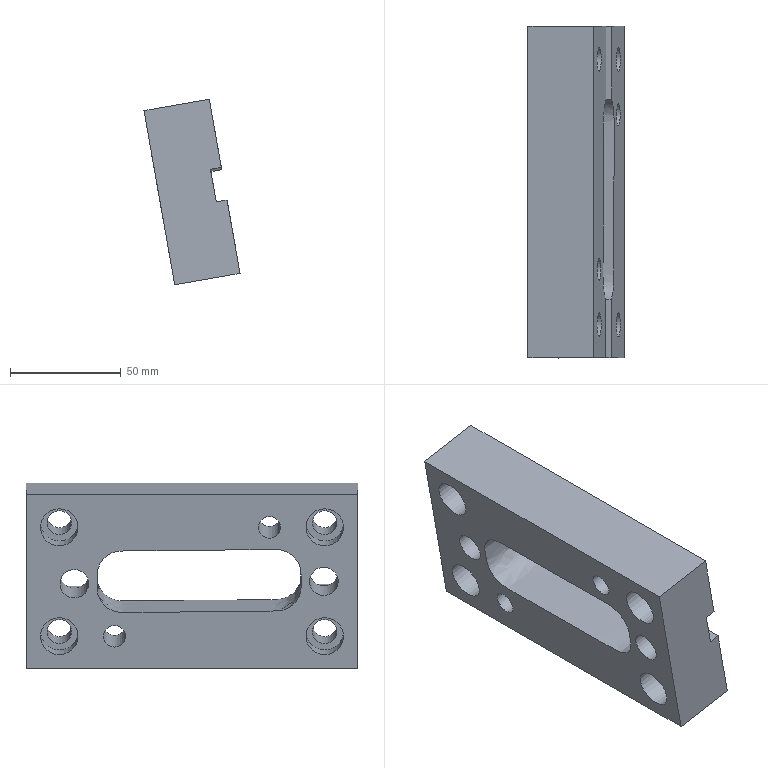Part | NX | features solid 2 | 1 solid | 30 faces | box 43.436 x 150 x 83.994 mm | volume 247913 mm3 | plane 17 | cylinder 12 | spline 1 | commonest cylinder face diameters 11 x4 17 x4 10 x2 13 x2